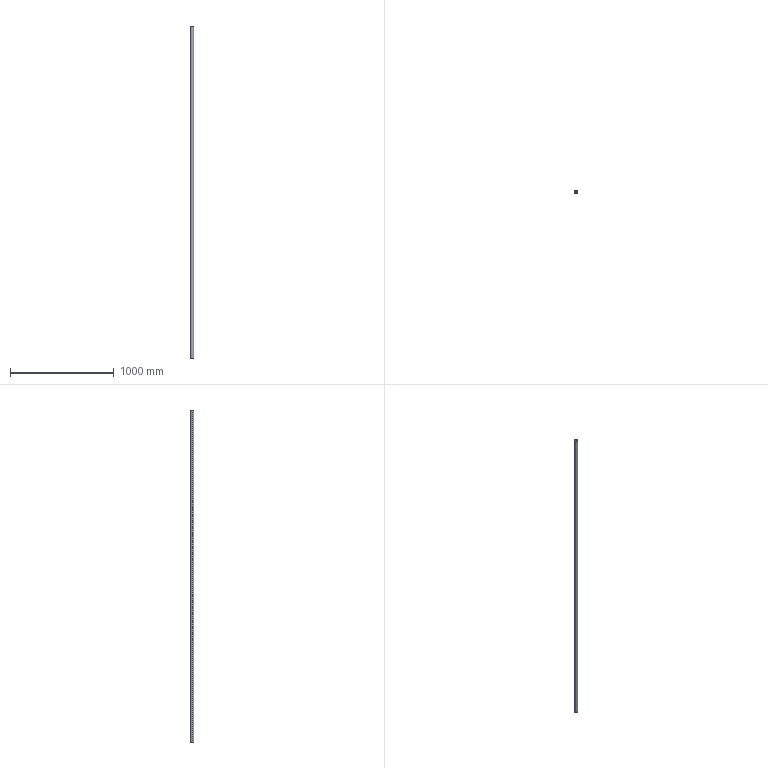Part | SolidWorks | features Extrusion 1 | 1 solid | 6 faces | box 32 x 32 x 3200 mm | volume 603186 mm3 | cylinder 4 | plane 2 | commonest cylinder face diameters 28 x2 32 x2
STEP:
#1=CARTESIAN_POINT('',(-14.,0.,1600.));
#2=VERTEX_POINT('',#1);
#3=CARTESIAN_POINT('',(14.,0.,1600.));
#4=VERTEX_POINT('',#3);
#5=CARTESIAN_POINT('',(0.,0.,1600.));
#6=DIRECTION('',(0.,0.,1.));
#7=DIRECTION('',(1.,0.,0.));
#8=AXIS2_PLACEMENT_3D('',#5,#6,#7);
#9=CIRCLE('',#8,14.);
#10=EDGE_CURVE('',#2,#4,#9,.T.);
#11=ORIENTED_EDGE('',*,*,#10,.T.);
#12=CARTESIAN_POINT('',(14.,0.,-1600.));
#13=VERTEX_POINT('',#12);
#14=CARTESIAN_POINT('',(14.,0.,1600.));
#15=DIRECTION('',(0.,0.,-1.));
#16=VECTOR('',#15,1000.);
#17=LINE('',#14,#16);
#18=EDGE_CURVE('',#4,#13,#17,.T.);
#19=ORIENTED_EDGE('',*,*,#18,.T.);
#20=CARTESIAN_POINT('',(-14.,0.,-1600.));
#21=VERTEX_POINT('',#20);
#22=CARTESIAN_POINT('',(0.,0.,-1600.));
#23=DIRECTION('',(0.,0.,1.));
#24=DIRECTION('',(1.,0.,0.));
#25=AXIS2_PLACEMENT_3D('',#22,#23,#24);
#26=CIRCLE('',#25,14.);
#27=EDGE_CURVE('',#21,#13,#26,.T.);
#28=ORIENTED_EDGE('',*,*,#27,.F.);
#29=CARTESIAN_POINT('',(-14.,0.,1600.));
#30=DIRECTION('',(0.,0.,-1.));
#31=VECTOR('',#30,1000.);
#32=LINE('',#29,#31);
#33=EDGE_CURVE('',#2,#21,#32,.T.);
#34=ORIENTED_EDGE('',*,*,#33,.F.);
#35=EDGE_LOOP('',(#11,#19,#28,#34));
#36=FACE_OUTER_BOUND('',#35,.T.);
#37=CARTESIAN_POINT('',(0.,0.,1600.));
#38=DIRECTION('',(0.,0.,-1.));
#39=DIRECTION('',(-1.,0.,0.));
#40=AXIS2_PLACEMENT_3D('',#37,#38,#39);
#41=CYLINDRICAL_SURFACE('',#40,14.);
#42=ADVANCED_FACE('',(#36),#41,.F.);
#43=CARTESIAN_POINT('',(16.,0.,1600.));
#44=VERTEX_POINT('',#43);
#45=CARTESIAN_POINT('',(-16.,0.,1600.));
#46=VERTEX_POINT('',#45);
#47=CARTESIAN_POINT('',(0.,0.,1600.));
#48=DIRECTION('',(0.,0.,1.));
#49=DIRECTION('',(1.,0.,0.));
#50=AXIS2_PLACEMENT_3D('',#47,#48,#49);
#51=CIRCLE('',#50,16.);
#52=EDGE_CURVE('',#44,#46,#51,.T.);
#53=ORIENTED_EDGE('',*,*,#52,.F.);
#54=CARTESIAN_POINT('',(16.,0.,-1600.));
#55=VERTEX_POINT('',#54);
#56=CARTESIAN_POINT('',(16.,0.,1600.));
#57=DIRECTION('',(0.,0.,-1.));
#58=VECTOR('',#57,1000.);
#59=LINE('',#56,#58);
#60=EDGE_CURVE('',#44,#55,#59,.T.);
#61=ORIENTED_EDGE('',*,*,#60,.T.);
#62=CARTESIAN_POINT('',(-16.,0.,-1600.));
#63=VERTEX_POINT('',#62);
#64=CARTESIAN_POINT('',(0.,0.,-1600.));
#65=DIRECTION('',(0.,0.,1.));
#66=DIRECTION('',(1.,0.,0.));
#67=AXIS2_PLACEMENT_3D('',#64,#65,#66);
#68=CIRCLE('',#67,16.);
#69=EDGE_CURVE('',#55,#63,#68,.T.);
#70=ORIENTED_EDGE('',*,*,#69,.T.);
#71=CARTESIAN_POINT('',(-16.,0.,1600.));
#72=DIRECTION('',(0.,0.,-1.));
#73=VECTOR('',#72,1000.);
#74=LINE('',#71,#73);
#75=EDGE_CURVE('',#46,#63,#74,.T.);
#76=ORIENTED_EDGE('',*,*,#75,.F.);
#77=EDGE_LOOP('',(#53,#61,#70,#76));
#78=FACE_OUTER_BOUND('',#77,.T.);
#79=CARTESIAN_POINT('',(0.,0.,1600.));
#80=DIRECTION('',(0.,0.,-1.));
#81=DIRECTION('',(-1.,0.,0.));
#82=AXIS2_PLACEMENT_3D('',#79,#80,#81);
#83=CYLINDRICAL_SURFACE('',#82,16.);
#84=ADVANCED_FACE('',(#78),#83,.T.);
#85=CARTESIAN_POINT('',(0.,0.,1600.));
#86=DIRECTION('',(0.,0.,1.));
#87=DIRECTION('',(1.,0.,0.));
#88=AXIS2_PLACEMENT_3D('',#85,#86,#87);
#89=CIRCLE('',#88,16.);
#90=EDGE_CURVE('',#46,#44,#89,.T.);
#91=ORIENTED_EDGE('',*,*,#90,.T.);
#92=ORIENTED_EDGE('',*,*,#52,.T.);
#93=EDGE_LOOP('',(#91,#92));
#94=FACE_OUTER_BOUND('',#93,.T.);
#95=ORIENTED_EDGE('',*,*,#10,.F.);
#96=CARTESIAN_POINT('',(0.,0.,1600.));
#97=DIRECTION('',(0.,0.,1.));
#98=DIRECTION('',(1.,0.,0.));
#99=AXIS2_PLACEMENT_3D('',#96,#97,#98);
#100=CIRCLE('',#99,14.);
#101=EDGE_CURVE('',#4,#2,#100,.T.);
#102=ORIENTED_EDGE('',*,*,#101,.F.);
#103=EDGE_LOOP('',(#95,#102));
#104=FACE_BOUND('',#103,.T.);
#105=CARTESIAN_POINT('',(0.,0.,1600.));
#106=DIRECTION('',(0.,0.,1.));
#107=DIRECTION('',(1.,0.,0.));
#108=AXIS2_PLACEMENT_3D('',#105,#106,#107);
#109=PLANE('',#108);
#110=ADVANCED_FACE('',(#94,#104),#109,.T.);
#111=CARTESIAN_POINT('',(0.,0.,-1600.));
#112=DIRECTION('',(0.,0.,1.));
#113=DIRECTION('',(1.,0.,0.));
#114=AXIS2_PLACEMENT_3D('',#111,#112,#113);
#115=CIRCLE('',#114,16.);
#116=EDGE_CURVE('',#63,#55,#115,.T.);
#117=ORIENTED_EDGE('',*,*,#116,.F.);
#118=ORIENTED_EDGE('',*,*,#69,.F.);
#119=EDGE_LOOP('',(#117,#118));
#120=FACE_OUTER_BOUND('',#119,.T.);
#121=ORIENTED_EDGE('',*,*,#27,.T.);
#122=CARTESIAN_POINT('',(0.,0.,-1600.));
#123=DIRECTION('',(0.,0.,1.));
#124=DIRECTION('',(1.,0.,0.));
#125=AXIS2_PLACEMENT_3D('',#122,#123,#124);
#126=CIRCLE('',#125,14.);
#127=EDGE_CURVE('',#13,#21,#126,.T.);
#128=ORIENTED_EDGE('',*,*,#127,.T.);
#129=EDGE_LOOP('',(#121,#128));
#130=FACE_BOUND('',#129,.T.);
#131=CARTESIAN_POINT('',(0.,0.,-1600.));
#132=DIRECTION('',(0.,0.,1.));
#133=DIRECTION('',(1.,0.,0.));
#134=AXIS2_PLACEMENT_3D('',#131,#132,#133);
#135=PLANE('',#134);
#136=ADVANCED_FACE('',(#120,#130),#135,.F.);
#137=ORIENTED_EDGE('',*,*,#60,.F.);
#138=ORIENTED_EDGE('',*,*,#90,.F.);
#139=ORIENTED_EDGE('',*,*,#75,.T.);
#140=ORIENTED_EDGE('',*,*,#116,.T.);
#141=EDGE_LOOP('',(#137,#138,#139,#140));
#142=FACE_OUTER_BOUND('',#141,.T.);
#143=CARTESIAN_POINT('',(0.,0.,1600.));
#144=DIRECTION('',(0.,0.,-1.));
#145=DIRECTION('',(-1.,0.,0.));
#146=AXIS2_PLACEMENT_3D('',#143,#144,#145);
#147=CYLINDRICAL_SURFACE('',#146,16.);
#148=ADVANCED_FACE('',(#142),#147,.T.);
#149=ORIENTED_EDGE('',*,*,#18,.F.);
#150=ORIENTED_EDGE('',*,*,#101,.T.);
#151=ORIENTED_EDGE('',*,*,#33,.T.);
#152=ORIENTED_EDGE('',*,*,#127,.F.);
#153=EDGE_LOOP('',(#149,#150,#151,#152));
#154=FACE_OUTER_BOUND('',#153,.T.);
#155=CARTESIAN_POINT('',(0.,0.,1600.));
#156=DIRECTION('',(0.,0.,-1.));
#157=DIRECTION('',(-1.,0.,0.));
#158=AXIS2_PLACEMENT_3D('',#155,#156,#157);
#159=CYLINDRICAL_SURFACE('',#158,14.);
#160=ADVANCED_FACE('',(#154),#159,.F.);
#161=CLOSED_SHELL('',(#42,#84,#110,#136,#148,#160));
#162=MANIFOLD_SOLID_BREP('',#161);
#163=CARTESIAN_POINT('',(0.,0.,0.));
#164=DIRECTION('',(0.,0.,1.));
#165=DIRECTION('',(1.,0.,0.));
#166=AXIS2_PLACEMENT_3D('',#163,#164,#165);
#167=(LENGTH_UNIT()NAMED_UNIT(*)SI_UNIT(.MILLI.,.METRE.));
#168=UNCERTAINTY_MEASURE_WITH_UNIT(LENGTH_MEASURE(0.00001),#167,'','');
#169=(NAMED_UNIT(*)PLANE_ANGLE_UNIT()SI_UNIT($,.RADIAN.));
#170=(NAMED_UNIT(*)SI_UNIT($,.STERADIAN.)SOLID_ANGLE_UNIT());
#171=(GEOMETRIC_REPRESENTATION_CONTEXT(3)GLOBAL_UNCERTAINTY_ASSIGNED_CONTEXT((#168))GLOBAL_UNIT_ASSIGNED_CONTEXT((#167,#169,#170))REPRESENTATION_CONTEXT('',''));
#172=ADVANCED_BREP_SHAPE_REPRESENTATION('',(#162,#166),#171);